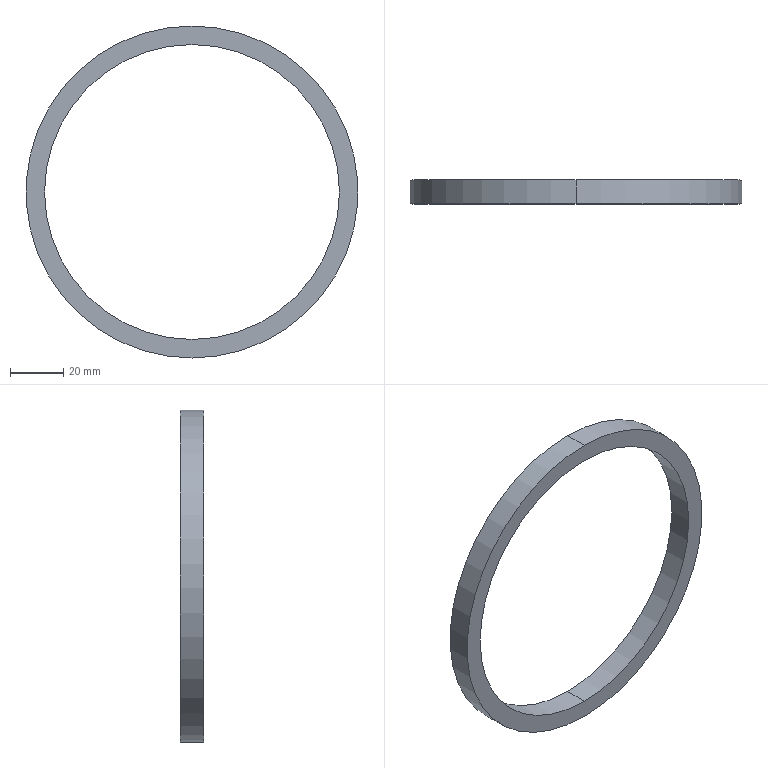Part | SolidWorks | features BaseBody 1 | 1 solid | 6 faces | box 125 x 9 x 125 mm | volume 23355 mm3 | cylinder 4 | plane 2 | commonest cylinder face diameters 111 x2 125 x2
STEP:
#1=CARTESIAN_POINT('',(0.,9.,55.5));
#2=VERTEX_POINT('',#1);
#3=CARTESIAN_POINT('',(0.,9.,-55.5));
#4=VERTEX_POINT('',#3);
#5=CARTESIAN_POINT('',(0.,9.,0.));
#6=DIRECTION('',(0.,-1.,0.));
#7=DIRECTION('',(0.,0.,-1.));
#8=AXIS2_PLACEMENT_3D('',#5,#6,#7);
#9=CIRCLE('',#8,55.5);
#10=EDGE_CURVE('',#2,#4,#9,.T.);
#11=ORIENTED_EDGE('',*,*,#10,.F.);
#12=CARTESIAN_POINT('',(0.,0.,55.5));
#13=VERTEX_POINT('',#12);
#14=CARTESIAN_POINT('',(0.,9.,55.5));
#15=DIRECTION('',(0.,-1.,0.));
#16=VECTOR('',#15,1000.);
#17=LINE('',#14,#16);
#18=EDGE_CURVE('',#2,#13,#17,.T.);
#19=ORIENTED_EDGE('',*,*,#18,.T.);
#20=CARTESIAN_POINT('',(0.,0.,-55.5));
#21=VERTEX_POINT('',#20);
#22=CARTESIAN_POINT('',(0.,0.,0.));
#23=DIRECTION('',(0.,1.,0.));
#24=DIRECTION('',(0.,0.,-1.));
#25=AXIS2_PLACEMENT_3D('',#22,#23,#24);
#26=CIRCLE('',#25,55.5);
#27=EDGE_CURVE('',#21,#13,#26,.T.);
#28=ORIENTED_EDGE('',*,*,#27,.F.);
#29=CARTESIAN_POINT('',(0.,9.,-55.5));
#30=DIRECTION('',(0.,-1.,0.));
#31=VECTOR('',#30,1000.);
#32=LINE('',#29,#31);
#33=EDGE_CURVE('',#4,#21,#32,.T.);
#34=ORIENTED_EDGE('',*,*,#33,.F.);
#35=EDGE_LOOP('',(#11,#19,#28,#34));
#36=FACE_OUTER_BOUND('',#35,.T.);
#37=CARTESIAN_POINT('',(0.,9.,0.));
#38=DIRECTION('',(0.,-1.,0.));
#39=DIRECTION('',(0.,0.,-1.));
#40=AXIS2_PLACEMENT_3D('',#37,#38,#39);
#41=CYLINDRICAL_SURFACE('',#40,55.5);
#42=ADVANCED_FACE('',(#36),#41,.F.);
#43=CARTESIAN_POINT('',(0.,9.,62.5));
#44=VERTEX_POINT('',#43);
#45=CARTESIAN_POINT('',(0.,9.,-62.5));
#46=VERTEX_POINT('',#45);
#47=CARTESIAN_POINT('',(0.,9.,0.));
#48=DIRECTION('',(0.,1.,0.));
#49=DIRECTION('',(0.,0.,-1.));
#50=AXIS2_PLACEMENT_3D('',#47,#48,#49);
#51=CIRCLE('',#50,62.5);
#52=EDGE_CURVE('',#44,#46,#51,.T.);
#53=ORIENTED_EDGE('',*,*,#52,.F.);
#54=CARTESIAN_POINT('',(0.,0.,62.5));
#55=VERTEX_POINT('',#54);
#56=CARTESIAN_POINT('',(0.,9.,62.5));
#57=DIRECTION('',(0.,-1.,0.));
#58=VECTOR('',#57,1000.);
#59=LINE('',#56,#58);
#60=EDGE_CURVE('',#44,#55,#59,.T.);
#61=ORIENTED_EDGE('',*,*,#60,.T.);
#62=CARTESIAN_POINT('',(0.,0.,-62.5));
#63=VERTEX_POINT('',#62);
#64=CARTESIAN_POINT('',(0.,0.,0.));
#65=DIRECTION('',(0.,1.,0.));
#66=DIRECTION('',(0.,0.,-1.));
#67=AXIS2_PLACEMENT_3D('',#64,#65,#66);
#68=CIRCLE('',#67,62.5);
#69=EDGE_CURVE('',#55,#63,#68,.T.);
#70=ORIENTED_EDGE('',*,*,#69,.T.);
#71=CARTESIAN_POINT('',(0.,9.,-62.5));
#72=DIRECTION('',(0.,-1.,0.));
#73=VECTOR('',#72,1000.);
#74=LINE('',#71,#73);
#75=EDGE_CURVE('',#46,#63,#74,.T.);
#76=ORIENTED_EDGE('',*,*,#75,.F.);
#77=EDGE_LOOP('',(#53,#61,#70,#76));
#78=FACE_OUTER_BOUND('',#77,.T.);
#79=CARTESIAN_POINT('',(0.,9.,0.));
#80=DIRECTION('',(0.,-1.,0.));
#81=DIRECTION('',(0.,0.,-1.));
#82=AXIS2_PLACEMENT_3D('',#79,#80,#81);
#83=CYLINDRICAL_SURFACE('',#82,62.5);
#84=ADVANCED_FACE('',(#78),#83,.T.);
#85=CARTESIAN_POINT('',(0.,9.,0.));
#86=DIRECTION('',(0.,-1.,0.));
#87=DIRECTION('',(0.,0.,-1.));
#88=AXIS2_PLACEMENT_3D('',#85,#86,#87);
#89=CIRCLE('',#88,55.5);
#90=EDGE_CURVE('',#4,#2,#89,.T.);
#91=ORIENTED_EDGE('',*,*,#90,.T.);
#92=ORIENTED_EDGE('',*,*,#10,.T.);
#93=EDGE_LOOP('',(#91,#92));
#94=FACE_BOUND('',#93,.T.);
#95=CARTESIAN_POINT('',(0.,9.,0.));
#96=DIRECTION('',(0.,1.,0.));
#97=DIRECTION('',(0.,0.,-1.));
#98=AXIS2_PLACEMENT_3D('',#95,#96,#97);
#99=CIRCLE('',#98,62.5);
#100=EDGE_CURVE('',#46,#44,#99,.T.);
#101=ORIENTED_EDGE('',*,*,#100,.T.);
#102=ORIENTED_EDGE('',*,*,#52,.T.);
#103=EDGE_LOOP('',(#101,#102));
#104=FACE_OUTER_BOUND('',#103,.T.);
#105=CARTESIAN_POINT('',(0.,9.,0.));
#106=DIRECTION('',(0.,1.,0.));
#107=DIRECTION('',(0.,0.,1.));
#108=AXIS2_PLACEMENT_3D('',#105,#106,#107);
#109=PLANE('',#108);
#110=ADVANCED_FACE('',(#94,#104),#109,.T.);
#111=ORIENTED_EDGE('',*,*,#18,.F.);
#112=ORIENTED_EDGE('',*,*,#90,.F.);
#113=ORIENTED_EDGE('',*,*,#33,.T.);
#114=CARTESIAN_POINT('',(0.,0.,0.));
#115=DIRECTION('',(0.,1.,0.));
#116=DIRECTION('',(0.,0.,-1.));
#117=AXIS2_PLACEMENT_3D('',#114,#115,#116);
#118=CIRCLE('',#117,55.5);
#119=EDGE_CURVE('',#13,#21,#118,.T.);
#120=ORIENTED_EDGE('',*,*,#119,.F.);
#121=EDGE_LOOP('',(#111,#112,#113,#120));
#122=FACE_OUTER_BOUND('',#121,.T.);
#123=CARTESIAN_POINT('',(0.,9.,0.));
#124=DIRECTION('',(0.,-1.,0.));
#125=DIRECTION('',(0.,0.,-1.));
#126=AXIS2_PLACEMENT_3D('',#123,#124,#125);
#127=CYLINDRICAL_SURFACE('',#126,55.5);
#128=ADVANCED_FACE('',(#122),#127,.F.);
#129=ORIENTED_EDGE('',*,*,#60,.F.);
#130=ORIENTED_EDGE('',*,*,#100,.F.);
#131=ORIENTED_EDGE('',*,*,#75,.T.);
#132=CARTESIAN_POINT('',(0.,0.,0.));
#133=DIRECTION('',(0.,1.,0.));
#134=DIRECTION('',(0.,0.,-1.));
#135=AXIS2_PLACEMENT_3D('',#132,#133,#134);
#136=CIRCLE('',#135,62.5);
#137=EDGE_CURVE('',#63,#55,#136,.T.);
#138=ORIENTED_EDGE('',*,*,#137,.T.);
#139=EDGE_LOOP('',(#129,#130,#131,#138));
#140=FACE_OUTER_BOUND('',#139,.T.);
#141=CARTESIAN_POINT('',(0.,9.,0.));
#142=DIRECTION('',(0.,-1.,0.));
#143=DIRECTION('',(0.,0.,-1.));
#144=AXIS2_PLACEMENT_3D('',#141,#142,#143);
#145=CYLINDRICAL_SURFACE('',#144,62.5);
#146=ADVANCED_FACE('',(#140),#145,.T.);
#147=ORIENTED_EDGE('',*,*,#27,.T.);
#148=ORIENTED_EDGE('',*,*,#119,.T.);
#149=EDGE_LOOP('',(#147,#148));
#150=FACE_BOUND('',#149,.T.);
#151=ORIENTED_EDGE('',*,*,#137,.F.);
#152=ORIENTED_EDGE('',*,*,#69,.F.);
#153=EDGE_LOOP('',(#151,#152));
#154=FACE_OUTER_BOUND('',#153,.T.);
#155=CARTESIAN_POINT('',(0.,0.,0.));
#156=DIRECTION('',(0.,1.,0.));
#157=DIRECTION('',(0.,0.,1.));
#158=AXIS2_PLACEMENT_3D('',#155,#156,#157);
#159=PLANE('',#158);
#160=ADVANCED_FACE('',(#150,#154),#159,.F.);
#161=CLOSED_SHELL('',(#42,#84,#110,#128,#146,#160));
#162=MANIFOLD_SOLID_BREP('',#161);
#163=CARTESIAN_POINT('',(0.,0.,0.));
#164=DIRECTION('',(0.,0.,1.));
#165=DIRECTION('',(1.,0.,0.));
#166=AXIS2_PLACEMENT_3D('',#163,#164,#165);
#167=(LENGTH_UNIT()NAMED_UNIT(*)SI_UNIT(.MILLI.,.METRE.));
#168=UNCERTAINTY_MEASURE_WITH_UNIT(LENGTH_MEASURE(0.00001),#167,'','');
#169=(NAMED_UNIT(*)PLANE_ANGLE_UNIT()SI_UNIT($,.RADIAN.));
#170=(NAMED_UNIT(*)SI_UNIT($,.STERADIAN.)SOLID_ANGLE_UNIT());
#171=(GEOMETRIC_REPRESENTATION_CONTEXT(3)GLOBAL_UNCERTAINTY_ASSIGNED_CONTEXT((#168))GLOBAL_UNIT_ASSIGNED_CONTEXT((#167,#169,#170))REPRESENTATION_CONTEXT('',''));
#172=ADVANCED_BREP_SHAPE_REPRESENTATION('',(#162,#166),#171);